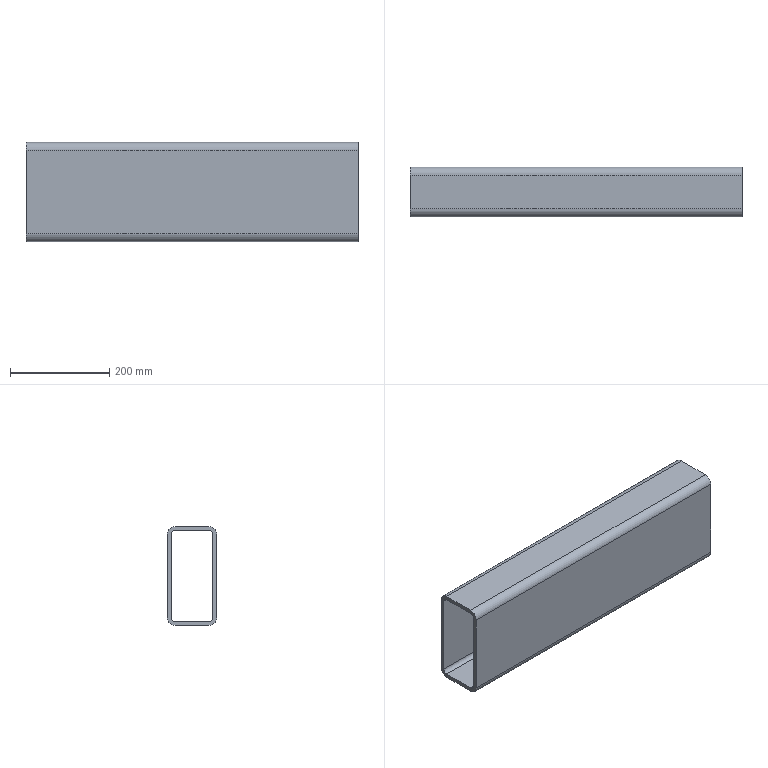Part | STEP file | 03-Longitudinal beam (flat tube 200x100x8)_default<machining> | 1 solid | 18 faces | box 670 x 100 x 200 mm | volume 2934054 mm3 | plane 10 | cylinder 8 | commonest cylinder face diameters 16 x4 32 x4
STEP:
#1=CARTESIAN_POINT('',(0.,0.,0.));
#2=DIRECTION('',(0.,0.,1.));
#3=DIRECTION('',(1.,0.,0.));
#4=AXIS2_PLACEMENT_3D('',#1,#2,#3);
#5=CARTESIAN_POINT('',(0.,50.,84.));
#6=VERTEX_POINT('',#5);
#7=CARTESIAN_POINT('',(0.,34.,100.));
#8=VERTEX_POINT('',#7);
#9=CARTESIAN_POINT('',(0.,34.,84.));
#10=DIRECTION('',(1.,0.,0.));
#11=DIRECTION('',(0.,0.,-1.));
#12=AXIS2_PLACEMENT_3D('',#9,#10,#11);
#13=CIRCLE('',#12,16.);
#14=CARTESIAN_POINT('',(670.,34.,84.));
#15=DIRECTION('',(-1.,0.,0.));
#16=DIRECTION('',(0.,0.,1.));
#17=AXIS2_PLACEMENT_3D('',#14,#15,#16);
#18=CYLINDRICAL_SURFACE('',#17,16.);
#19=CARTESIAN_POINT('',(3.142,670.));
#20=DIRECTION('',(-1.,0.));
#21=VECTOR('',#20,1.);
#22=LINE('',#19,#21);
#23=(GEOMETRIC_REPRESENTATION_CONTEXT(2)PARAMETRIC_REPRESENTATION_CONTEXT()REPRESENTATION_CONTEXT('',''));
#24=DEFINITIONAL_REPRESENTATION('',(#22),#23);
#25=PCURVE('',#18,#24);
#26=CARTESIAN_POINT('',(0.,34.,84.));
#27=DIRECTION('',(1.,0.,0.));
#28=DIRECTION('',(0.,0.,-1.));
#29=AXIS2_PLACEMENT_3D('',#26,#27,#28);
#30=PLANE('',#29);
#31=CARTESIAN_POINT('',(0.,0.));
#32=DIRECTION('',(1.,0.));
#33=AXIS2_PLACEMENT_2D('',#31,#32);
#34=CIRCLE('',#33,16.);
#35=(GEOMETRIC_REPRESENTATION_CONTEXT(2)PARAMETRIC_REPRESENTATION_CONTEXT()REPRESENTATION_CONTEXT('',''));
#36=DEFINITIONAL_REPRESENTATION('',(#34),#35);
#37=PCURVE('',#30,#36);
#38=SURFACE_CURVE('',#13,(#25,#37),.PCURVE_S1.);
#39=EDGE_CURVE('',#6,#8,#38,.T.);
#40=ORIENTED_EDGE('',*,*,#39,.T.);
#41=CARTESIAN_POINT('',(670.,34.,100.));
#42=VERTEX_POINT('',#41);
#43=CARTESIAN_POINT('',(670.,34.,100.));
#44=DIRECTION('',(-1.,0.,0.));
#45=VECTOR('',#44,1.);
#46=LINE('',#43,#45);
#47=CARTESIAN_POINT('',(0.,0.));
#48=DIRECTION('',(0.,1.));
#49=VECTOR('',#48,1.);
#50=LINE('',#47,#49);
#51=(GEOMETRIC_REPRESENTATION_CONTEXT(2)PARAMETRIC_REPRESENTATION_CONTEXT()REPRESENTATION_CONTEXT('',''));
#52=DEFINITIONAL_REPRESENTATION('',(#50),#51);
#53=PCURVE('',#18,#52);
#54=CARTESIAN_POINT('',(670.,34.,100.));
#55=DIRECTION('',(0.,0.,-1.));
#56=DIRECTION('',(-1.,0.,0.));
#57=AXIS2_PLACEMENT_3D('',#54,#55,#56);
#58=PLANE('',#57);
#59=CARTESIAN_POINT('',(0.,0.));
#60=DIRECTION('',(1.,0.));
#61=VECTOR('',#60,1.);
#62=LINE('',#59,#61);
#63=(GEOMETRIC_REPRESENTATION_CONTEXT(2)PARAMETRIC_REPRESENTATION_CONTEXT()REPRESENTATION_CONTEXT('',''));
#64=DEFINITIONAL_REPRESENTATION('',(#62),#63);
#65=PCURVE('',#58,#64);
#66=SURFACE_CURVE('',#46,(#53,#65),.PCURVE_S1.);
#67=EDGE_CURVE('',#42,#8,#66,.T.);
#68=ORIENTED_EDGE('',*,*,#67,.F.);
#69=CARTESIAN_POINT('',(670.,50.,84.));
#70=VERTEX_POINT('',#69);
#71=CARTESIAN_POINT('',(670.,34.,84.));
#72=DIRECTION('',(1.,0.,0.));
#73=DIRECTION('',(0.,0.,-1.));
#74=AXIS2_PLACEMENT_3D('',#71,#72,#73);
#75=CIRCLE('',#74,16.);
#76=CARTESIAN_POINT('',(3.142,0.));
#77=DIRECTION('',(-1.,0.));
#78=VECTOR('',#77,1.);
#79=LINE('',#76,#78);
#80=(GEOMETRIC_REPRESENTATION_CONTEXT(2)PARAMETRIC_REPRESENTATION_CONTEXT()REPRESENTATION_CONTEXT('',''));
#81=DEFINITIONAL_REPRESENTATION('',(#79),#80);
#82=PCURVE('',#18,#81);
#83=CARTESIAN_POINT('',(670.,34.,84.));
#84=DIRECTION('',(1.,0.,0.));
#85=DIRECTION('',(0.,0.,-1.));
#86=AXIS2_PLACEMENT_3D('',#83,#84,#85);
#87=PLANE('',#86);
#88=CARTESIAN_POINT('',(0.,0.));
#89=DIRECTION('',(1.,0.));
#90=AXIS2_PLACEMENT_2D('',#88,#89);
#91=CIRCLE('',#90,16.);
#92=(GEOMETRIC_REPRESENTATION_CONTEXT(2)PARAMETRIC_REPRESENTATION_CONTEXT()REPRESENTATION_CONTEXT('',''));
#93=DEFINITIONAL_REPRESENTATION('',(#91),#92);
#94=PCURVE('',#87,#93);
#95=SURFACE_CURVE('',#75,(#82,#94),.PCURVE_S1.);
#96=EDGE_CURVE('',#70,#42,#95,.T.);
#97=ORIENTED_EDGE('',*,*,#96,.F.);
#98=CARTESIAN_POINT('',(670.,50.,84.));
#99=DIRECTION('',(-1.,0.,0.));
#100=VECTOR('',#99,1.);
#101=LINE('',#98,#100);
#102=CARTESIAN_POINT('',(1.571,0.));
#103=DIRECTION('',(0.,1.));
#104=VECTOR('',#103,1.);
#105=LINE('',#102,#104);
#106=(GEOMETRIC_REPRESENTATION_CONTEXT(2)PARAMETRIC_REPRESENTATION_CONTEXT()REPRESENTATION_CONTEXT('',''));
#107=DEFINITIONAL_REPRESENTATION('',(#105),#106);
#108=PCURVE('',#18,#107);
#109=CARTESIAN_POINT('',(670.,50.,84.));
#110=DIRECTION('',(0.,-1.,0.));
#111=DIRECTION('',(0.,0.,-1.));
#112=AXIS2_PLACEMENT_3D('',#109,#110,#111);
#113=PLANE('',#112);
#114=CARTESIAN_POINT('',(0.,0.));
#115=DIRECTION('',(0.,-1.));
#116=VECTOR('',#115,1.);
#117=LINE('',#114,#116);
#118=(GEOMETRIC_REPRESENTATION_CONTEXT(2)PARAMETRIC_REPRESENTATION_CONTEXT()REPRESENTATION_CONTEXT('',''));
#119=DEFINITIONAL_REPRESENTATION('',(#117),#118);
#120=PCURVE('',#113,#119);
#121=SURFACE_CURVE('',#101,(#108,#120),.PCURVE_S1.);
#122=EDGE_CURVE('',#70,#6,#121,.T.);
#123=ORIENTED_EDGE('',*,*,#122,.T.);
#124=EDGE_LOOP('',(#40,#68,#97,#123));
#125=FACE_BOUND('',#124,.T.);
#126=ADVANCED_FACE('',(#125),#18,.T.);
#127=CARTESIAN_POINT('',(0.,-34.,100.));
#128=VERTEX_POINT('',#127);
#129=CARTESIAN_POINT('',(0.,34.,100.));
#130=DIRECTION('',(0.,-1.,0.));
#131=VECTOR('',#130,1.);
#132=LINE('',#129,#131);
#133=CARTESIAN_POINT('',(670.,0.));
#134=DIRECTION('',(0.,-1.));
#135=VECTOR('',#134,1.);
#136=LINE('',#133,#135);
#137=(GEOMETRIC_REPRESENTATION_CONTEXT(2)PARAMETRIC_REPRESENTATION_CONTEXT()REPRESENTATION_CONTEXT('',''));
#138=DEFINITIONAL_REPRESENTATION('',(#136),#137);
#139=PCURVE('',#58,#138);
#140=CARTESIAN_POINT('',(-16.,0.));
#141=DIRECTION('',(0.,-1.));
#142=VECTOR('',#141,1.);
#143=LINE('',#140,#142);
#144=(GEOMETRIC_REPRESENTATION_CONTEXT(2)PARAMETRIC_REPRESENTATION_CONTEXT()REPRESENTATION_CONTEXT('',''));
#145=DEFINITIONAL_REPRESENTATION('',(#143),#144);
#146=PCURVE('',#30,#145);
#147=SURFACE_CURVE('',#132,(#139,#146),.PCURVE_S1.);
#148=EDGE_CURVE('',#8,#128,#147,.T.);
#149=ORIENTED_EDGE('',*,*,#148,.T.);
#150=CARTESIAN_POINT('',(670.,-34.,100.));
#151=VERTEX_POINT('',#150);
#152=CARTESIAN_POINT('',(670.,-34.,100.));
#153=DIRECTION('',(-1.,0.,0.));
#154=VECTOR('',#153,1.);
#155=LINE('',#152,#154);
#156=CARTESIAN_POINT('',(0.,-68.));
#157=DIRECTION('',(1.,0.));
#158=VECTOR('',#157,1.);
#159=LINE('',#156,#158);
#160=(GEOMETRIC_REPRESENTATION_CONTEXT(2)PARAMETRIC_REPRESENTATION_CONTEXT()REPRESENTATION_CONTEXT('',''));
#161=DEFINITIONAL_REPRESENTATION('',(#159),#160);
#162=PCURVE('',#58,#161);
#163=CARTESIAN_POINT('',(670.,-34.,84.));
#164=DIRECTION('',(-1.,0.,0.));
#165=DIRECTION('',(0.,0.,1.));
#166=AXIS2_PLACEMENT_3D('',#163,#164,#165);
#167=CYLINDRICAL_SURFACE('',#166,16.);
#168=CARTESIAN_POINT('',(6.283,0.));
#169=DIRECTION('',(0.,1.));
#170=VECTOR('',#169,1.);
#171=LINE('',#168,#170);
#172=(GEOMETRIC_REPRESENTATION_CONTEXT(2)PARAMETRIC_REPRESENTATION_CONTEXT()REPRESENTATION_CONTEXT('',''));
#173=DEFINITIONAL_REPRESENTATION('',(#171),#172);
#174=PCURVE('',#167,#173);
#175=SURFACE_CURVE('',#155,(#162,#174),.PCURVE_S1.);
#176=EDGE_CURVE('',#151,#128,#175,.T.);
#177=ORIENTED_EDGE('',*,*,#176,.F.);
#178=CARTESIAN_POINT('',(670.,34.,100.));
#179=DIRECTION('',(0.,-1.,0.));
#180=VECTOR('',#179,1.);
#181=LINE('',#178,#180);
#182=CARTESIAN_POINT('',(0.,0.));
#183=DIRECTION('',(0.,-1.));
#184=VECTOR('',#183,1.);
#185=LINE('',#182,#184);
#186=(GEOMETRIC_REPRESENTATION_CONTEXT(2)PARAMETRIC_REPRESENTATION_CONTEXT()REPRESENTATION_CONTEXT('',''));
#187=DEFINITIONAL_REPRESENTATION('',(#185),#186);
#188=PCURVE('',#58,#187);
#189=CARTESIAN_POINT('',(-16.,0.));
#190=DIRECTION('',(0.,-1.));
#191=VECTOR('',#190,1.);
#192=LINE('',#189,#191);
#193=(GEOMETRIC_REPRESENTATION_CONTEXT(2)PARAMETRIC_REPRESENTATION_CONTEXT()REPRESENTATION_CONTEXT('',''));
#194=DEFINITIONAL_REPRESENTATION('',(#192),#193);
#195=PCURVE('',#87,#194);
#196=SURFACE_CURVE('',#181,(#188,#195),.PCURVE_S1.);
#197=EDGE_CURVE('',#42,#151,#196,.T.);
#198=ORIENTED_EDGE('',*,*,#197,.F.);
#199=ORIENTED_EDGE('',*,*,#67,.T.);
#200=EDGE_LOOP('',(#149,#177,#198,#199));
#201=FACE_BOUND('',#200,.T.);
#202=ADVANCED_FACE('',(#201),#58,.F.);
#203=CARTESIAN_POINT('',(0.,-50.,84.));
#204=VERTEX_POINT('',#203);
#205=CARTESIAN_POINT('',(0.,-34.,84.));
#206=DIRECTION('',(1.,0.,0.));
#207=DIRECTION('',(0.,0.,-1.));
#208=AXIS2_PLACEMENT_3D('',#205,#206,#207);
#209=CIRCLE('',#208,16.);
#210=CARTESIAN_POINT('',(9.425,670.));
#211=DIRECTION('',(-1.,0.));
#212=VECTOR('',#211,1.);
#213=LINE('',#210,#212);
#214=(GEOMETRIC_REPRESENTATION_CONTEXT(2)PARAMETRIC_REPRESENTATION_CONTEXT()REPRESENTATION_CONTEXT('',''));
#215=DEFINITIONAL_REPRESENTATION('',(#213),#214);
#216=PCURVE('',#167,#215);
#217=CARTESIAN_POINT('',(0.,-68.));
#218=DIRECTION('',(1.,0.));
#219=AXIS2_PLACEMENT_2D('',#217,#218);
#220=CIRCLE('',#219,16.);
#221=(GEOMETRIC_REPRESENTATION_CONTEXT(2)PARAMETRIC_REPRESENTATION_CONTEXT()REPRESENTATION_CONTEXT('',''));
#222=DEFINITIONAL_REPRESENTATION('',(#220),#221);
#223=PCURVE('',#30,#222);
#224=SURFACE_CURVE('',#209,(#216,#223),.PCURVE_S1.);
#225=EDGE_CURVE('',#128,#204,#224,.T.);
#226=ORIENTED_EDGE('',*,*,#225,.T.);
#227=CARTESIAN_POINT('',(670.,-50.,84.));
#228=VERTEX_POINT('',#227);
#229=CARTESIAN_POINT('',(670.,-50.,84.));
#230=DIRECTION('',(-1.,0.,0.));
#231=VECTOR('',#230,1.);
#232=LINE('',#229,#231);
#233=CARTESIAN_POINT('',(4.712,0.));
#234=DIRECTION('',(0.,1.));
#235=VECTOR('',#234,1.);
#236=LINE('',#233,#235);
#237=(GEOMETRIC_REPRESENTATION_CONTEXT(2)PARAMETRIC_REPRESENTATION_CONTEXT()REPRESENTATION_CONTEXT('',''));
#238=DEFINITIONAL_REPRESENTATION('',(#236),#237);
#239=PCURVE('',#167,#238);
#240=CARTESIAN_POINT('',(670.,-50.,-84.));
#241=DIRECTION('',(0.,1.,0.));
#242=DIRECTION('',(0.,0.,1.));
#243=AXIS2_PLACEMENT_3D('',#240,#241,#242);
#244=PLANE('',#243);
#245=CARTESIAN_POINT('',(168.,0.));
#246=DIRECTION('',(0.,-1.));
#247=VECTOR('',#246,1.);
#248=LINE('',#245,#247);
#249=(GEOMETRIC_REPRESENTATION_CONTEXT(2)PARAMETRIC_REPRESENTATION_CONTEXT()REPRESENTATION_CONTEXT('',''));
#250=DEFINITIONAL_REPRESENTATION('',(#248),#249);
#251=PCURVE('',#244,#250);
#252=SURFACE_CURVE('',#232,(#239,#251),.PCURVE_S1.);
#253=EDGE_CURVE('',#228,#204,#252,.T.);
#254=ORIENTED_EDGE('',*,*,#253,.F.);
#255=CARTESIAN_POINT('',(670.,-34.,84.));
#256=DIRECTION('',(1.,0.,0.));
#257=DIRECTION('',(0.,0.,-1.));
#258=AXIS2_PLACEMENT_3D('',#255,#256,#257);
#259=CIRCLE('',#258,16.);
#260=CARTESIAN_POINT('',(9.425,0.));
#261=DIRECTION('',(-1.,0.));
#262=VECTOR('',#261,1.);
#263=LINE('',#260,#262);
#264=(GEOMETRIC_REPRESENTATION_CONTEXT(2)PARAMETRIC_REPRESENTATION_CONTEXT()REPRESENTATION_CONTEXT('',''));
#265=DEFINITIONAL_REPRESENTATION('',(#263),#264);
#266=PCURVE('',#167,#265);
#267=CARTESIAN_POINT('',(0.,-68.));
#268=DIRECTION('',(1.,0.));
#269=AXIS2_PLACEMENT_2D('',#267,#268);
#270=CIRCLE('',#269,16.);
#271=(GEOMETRIC_REPRESENTATION_CONTEXT(2)PARAMETRIC_REPRESENTATION_CONTEXT()REPRESENTATION_CONTEXT('',''));
#272=DEFINITIONAL_REPRESENTATION('',(#270),#271);
#273=PCURVE('',#87,#272);
#274=SURFACE_CURVE('',#259,(#266,#273),.PCURVE_S1.);
#275=EDGE_CURVE('',#151,#228,#274,.T.);
#276=ORIENTED_EDGE('',*,*,#275,.F.);
#277=ORIENTED_EDGE('',*,*,#176,.T.);
#278=EDGE_LOOP('',(#226,#254,#276,#277));
#279=FACE_BOUND('',#278,.T.);
#280=ADVANCED_FACE('',(#279),#167,.T.);
#281=CARTESIAN_POINT('',(0.,-50.,-84.));
#282=VERTEX_POINT('',#281);
#283=CARTESIAN_POINT('',(0.,-50.,-84.));
#284=DIRECTION('',(0.,0.,-1.));
#285=VECTOR('',#284,1.);
#286=LINE('',#283,#285);
#287=CARTESIAN_POINT('',(0.,-670.));
#288=DIRECTION('',(-1.,0.));
#289=VECTOR('',#288,1.);
#290=LINE('',#287,#289);
#291=(GEOMETRIC_REPRESENTATION_CONTEXT(2)PARAMETRIC_REPRESENTATION_CONTEXT()REPRESENTATION_CONTEXT('',''));
#292=DEFINITIONAL_REPRESENTATION('',(#290),#291);
#293=PCURVE('',#244,#292);
#294=CARTESIAN_POINT('',(168.,-84.));
#295=DIRECTION('',(1.,0.));
#296=VECTOR('',#295,1.);
#297=LINE('',#294,#296);
#298=(GEOMETRIC_REPRESENTATION_CONTEXT(2)PARAMETRIC_REPRESENTATION_CONTEXT()REPRESENTATION_CONTEXT('',''));
#299=DEFINITIONAL_REPRESENTATION('',(#297),#298);
#300=PCURVE('',#30,#299);
#301=SURFACE_CURVE('',#286,(#293,#300),.PCURVE_S1.);
#302=EDGE_CURVE('',#204,#282,#301,.T.);
#303=ORIENTED_EDGE('',*,*,#302,.T.);
#304=CARTESIAN_POINT('',(670.,-50.,-84.));
#305=VERTEX_POINT('',#304);
#306=CARTESIAN_POINT('',(670.,-50.,-84.));
#307=DIRECTION('',(-1.,0.,0.));
#308=VECTOR('',#307,1.);
#309=LINE('',#306,#308);
#310=CARTESIAN_POINT('',(0.,0.));
#311=DIRECTION('',(0.,-1.));
#312=VECTOR('',#311,1.);
#313=LINE('',#310,#312);
#314=(GEOMETRIC_REPRESENTATION_CONTEXT(2)PARAMETRIC_REPRESENTATION_CONTEXT()REPRESENTATION_CONTEXT('',''));
#315=DEFINITIONAL_REPRESENTATION('',(#313),#314);
#316=PCURVE('',#244,#315);
#317=CARTESIAN_POINT('',(670.,-34.,-84.));
#318=DIRECTION('',(-1.,0.,0.));
#319=DIRECTION('',(0.,0.,1.));
#320=AXIS2_PLACEMENT_3D('',#317,#318,#319);
#321=CYLINDRICAL_SURFACE('',#320,16.);
#322=CARTESIAN_POINT('',(4.712,0.));
#323=DIRECTION('',(0.,1.));
#324=VECTOR('',#323,1.);
#325=LINE('',#322,#324);
#326=(GEOMETRIC_REPRESENTATION_CONTEXT(2)PARAMETRIC_REPRESENTATION_CONTEXT()REPRESENTATION_CONTEXT('',''));
#327=DEFINITIONAL_REPRESENTATION('',(#325),#326);
#328=PCURVE('',#321,#327);
#329=SURFACE_CURVE('',#309,(#316,#328),.PCURVE_S1.);
#330=EDGE_CURVE('',#305,#282,#329,.T.);
#331=ORIENTED_EDGE('',*,*,#330,.F.);
#332=CARTESIAN_POINT('',(670.,-50.,-84.));
#333=DIRECTION('',(0.,0.,-1.));
#334=VECTOR('',#333,1.);
#335=LINE('',#332,#334);
#336=CARTESIAN_POINT('',(0.,0.));
#337=DIRECTION('',(-1.,0.));
#338=VECTOR('',#337,1.);
#339=LINE('',#336,#338);
#340=(GEOMETRIC_REPRESENTATION_CONTEXT(2)PARAMETRIC_REPRESENTATION_CONTEXT()REPRESENTATION_CONTEXT('',''));
#341=DEFINITIONAL_REPRESENTATION('',(#339),#340);
#342=PCURVE('',#244,#341);
#343=CARTESIAN_POINT('',(168.,-84.));
#344=DIRECTION('',(1.,0.));
#345=VECTOR('',#344,1.);
#346=LINE('',#343,#345);
#347=(GEOMETRIC_REPRESENTATION_CONTEXT(2)PARAMETRIC_REPRESENTATION_CONTEXT()REPRESENTATION_CONTEXT('',''));
#348=DEFINITIONAL_REPRESENTATION('',(#346),#347);
#349=PCURVE('',#87,#348);
#350=SURFACE_CURVE('',#335,(#342,#349),.PCURVE_S1.);
#351=EDGE_CURVE('',#228,#305,#350,.T.);
#352=ORIENTED_EDGE('',*,*,#351,.F.);
#353=ORIENTED_EDGE('',*,*,#253,.T.);
#354=EDGE_LOOP('',(#303,#331,#352,#353));
#355=FACE_BOUND('',#354,.T.);
#356=ADVANCED_FACE('',(#355),#244,.F.);
#357=CARTESIAN_POINT('',(0.,-34.,-100.));
#358=VERTEX_POINT('',#357);
#359=CARTESIAN_POINT('',(0.,-34.,-84.));
#360=DIRECTION('',(1.,0.,0.));
#361=DIRECTION('',(0.,0.,-1.));
#362=AXIS2_PLACEMENT_3D('',#359,#360,#361);
#363=CIRCLE('',#362,16.);
#364=CARTESIAN_POINT('',(9.425,670.));
#365=DIRECTION('',(-1.,0.));
#366=VECTOR('',#365,1.);
#367=LINE('',#364,#366);
#368=(GEOMETRIC_REPRESENTATION_CONTEXT(2)PARAMETRIC_REPRESENTATION_CONTEXT()REPRESENTATION_CONTEXT('',''));
#369=DEFINITIONAL_REPRESENTATION('',(#367),#368);
#370=PCURVE('',#321,#369);
#371=CARTESIAN_POINT('',(168.,-68.));
#372=DIRECTION('',(1.,0.));
#373=AXIS2_PLACEMENT_2D('',#371,#372);
#374=CIRCLE('',#373,16.);
#375=(GEOMETRIC_REPRESENTATION_CONTEXT(2)PARAMETRIC_REPRESENTATION_CONTEXT()REPRESENTATION_CONTEXT('',''));
#376=DEFINITIONAL_REPRESENTATION('',(#374),#375);
#377=PCURVE('',#30,#376);
#378=SURFACE_CURVE('',#363,(#370,#377),.PCURVE_S1.);
#379=EDGE_CURVE('',#282,#358,#378,.T.);
#380=ORIENTED_EDGE('',*,*,#379,.T.);
#381=CARTESIAN_POINT('',(670.,-34.,-100.));
#382=VERTEX_POINT('',#381);
#383=CARTESIAN_POINT('',(670.,-34.,-100.));
#384=DIRECTION('',(-1.,0.,0.));
#385=VECTOR('',#384,1.);
#386=LINE('',#383,#385);
#387=CARTESIAN_POINT('',(3.142,0.));
#388=DIRECTION('',(0.,1.));
#389=VECTOR('',#388,1.);
#390=LINE('',#387,#389);
#391=(GEOMETRIC_REPRESENTATION_CONTEXT(2)PARAMETRIC_REPRESENTATION_CONTEXT()REPRESENTATION_CONTEXT('',''));
#392=DEFINITIONAL_REPRESENTATION('',(#390),#391);
#393=PCURVE('',#321,#392);
#394=CARTESIAN_POINT('',(670.,-34.,-100.));
#395=DIRECTION('',(0.,0.,1.));
#396=DIRECTION('',(1.,0.,0.));
#397=AXIS2_PLACEMENT_3D('',#394,#395,#396);
#398=PLANE('',#397);
#399=CARTESIAN_POINT('',(0.,0.));
#400=DIRECTION('',(-1.,0.));
#401=VECTOR('',#400,1.);
#402=LINE('',#399,#401);
#403=(GEOMETRIC_REPRESENTATION_CONTEXT(2)PARAMETRIC_REPRESENTATION_CONTEXT()REPRESENTATION_CONTEXT('',''));
#404=DEFINITIONAL_REPRESENTATION('',(#402),#403);
#405=PCURVE('',#398,#404);
#406=SURFACE_CURVE('',#386,(#393,#405),.PCURVE_S1.);
#407=EDGE_CURVE('',#382,#358,#406,.T.);
#408=ORIENTED_EDGE('',*,*,#407,.F.);
#409=CARTESIAN_POINT('',(670.,-34.,-84.));
#410=DIRECTION('',(1.,0.,0.));
#411=DIRECTION('',(0.,0.,-1.));
#412=AXIS2_PLACEMENT_3D('',#409,#410,#411);
#413=CIRCLE('',#412,16.);
#414=CARTESIAN_POINT('',(9.425,0.));
#415=DIRECTION('',(-1.,0.));
#416=VECTOR('',#415,1.);
#417=LINE('',#414,#416);
#418=(GEOMETRIC_REPRESENTATION_CONTEXT(2)PARAMETRIC_REPRESENTATION_CONTEXT()REPRESENTATION_CONTEXT('',''));
#419=DEFINITIONAL_REPRESENTATION('',(#417),#418);
#420=PCURVE('',#321,#419);
#421=CARTESIAN_POINT('',(168.,-68.));
#422=DIRECTION('',(1.,0.));
#423=AXIS2_PLACEMENT_2D('',#421,#422);
#424=CIRCLE('',#423,16.);
#425=(GEOMETRIC_REPRESENTATION_CONTEXT(2)PARAMETRIC_REPRESENTATION_CONTEXT()REPRESENTATION_CONTEXT('',''));
#426=DEFINITIONAL_REPRESENTATION('',(#424),#425);
#427=PCURVE('',#87,#426);
#428=SURFACE_CURVE('',#413,(#420,#427),.PCURVE_S1.);
#429=EDGE_CURVE('',#305,#382,#428,.T.);
#430=ORIENTED_EDGE('',*,*,#429,.F.);
#431=ORIENTED_EDGE('',*,*,#330,.T.);
#432=EDGE_LOOP('',(#380,#408,#430,#431));
#433=FACE_BOUND('',#432,.T.);
#434=ADVANCED_FACE('',(#433),#321,.T.);
#435=CARTESIAN_POINT('',(0.,34.,-100.));
#436=VERTEX_POINT('',#435);
#437=CARTESIAN_POINT('',(0.,-34.,-100.));
#438=DIRECTION('',(0.,1.,0.));
#439=VECTOR('',#438,1.);
#440=LINE('',#437,#439);
#441=CARTESIAN_POINT('',(-670.,0.));
#442=DIRECTION('',(0.,1.));
#443=VECTOR('',#442,1.);
#444=LINE('',#441,#443);
#445=(GEOMETRIC_REPRESENTATION_CONTEXT(2)PARAMETRIC_REPRESENTATION_CONTEXT()REPRESENTATION_CONTEXT('',''));
#446=DEFINITIONAL_REPRESENTATION('',(#444),#445);
#447=PCURVE('',#398,#446);
#448=CARTESIAN_POINT('',(184.,-68.));
#449=DIRECTION('',(0.,1.));
#450=VECTOR('',#449,1.);
#451=LINE('',#448,#450);
#452=(GEOMETRIC_REPRESENTATION_CONTEXT(2)PARAMETRIC_REPRESENTATION_CONTEXT()REPRESENTATION_CONTEXT('',''));
#453=DEFINITIONAL_REPRESENTATION('',(#451),#452);
#454=PCURVE('',#30,#453);
#455=SURFACE_CURVE('',#440,(#447,#454),.PCURVE_S1.);
#456=EDGE_CURVE('',#358,#436,#455,.T.);
#457=ORIENTED_EDGE('',*,*,#456,.T.);
#458=CARTESIAN_POINT('',(670.,34.,-100.));
#459=VERTEX_POINT('',#458);
#460=CARTESIAN_POINT('',(670.,34.,-100.));
#461=DIRECTION('',(-1.,0.,0.));
#462=VECTOR('',#461,1.);
#463=LINE('',#460,#462);
#464=CARTESIAN_POINT('',(0.,68.));
#465=DIRECTION('',(-1.,0.));
#466=VECTOR('',#465,1.);
#467=LINE('',#464,#466);
#468=(GEOMETRIC_REPRESENTATION_CONTEXT(2)PARAMETRIC_REPRESENTATION_CONTEXT()REPRESENTATION_CONTEXT('',''));
#469=DEFINITIONAL_REPRESENTATION('',(#467),#468);
#470=PCURVE('',#398,#469);
#471=CARTESIAN_POINT('',(670.,34.,-84.));
#472=DIRECTION('',(-1.,0.,0.));
#473=DIRECTION('',(0.,0.,1.));
#474=AXIS2_PLACEMENT_3D('',#471,#472,#473);
#475=CYLINDRICAL_SURFACE('',#474,16.);
#476=CARTESIAN_POINT('',(3.142,0.));
#477=DIRECTION('',(0.,1.));
#478=VECTOR('',#477,1.);
#479=LINE('',#476,#478);
#480=(GEOMETRIC_REPRESENTATION_CONTEXT(2)PARAMETRIC_REPRESENTATION_CONTEXT()REPRESENTATION_CONTEXT('',''));
#481=DEFINITIONAL_REPRESENTATION('',(#479),#480);
#482=PCURVE('',#475,#481);
#483=SURFACE_CURVE('',#463,(#470,#482),.PCURVE_S1.);
#484=EDGE_CURVE('',#459,#436,#483,.T.);
#485=ORIENTED_EDGE('',*,*,#484,.F.);
#486=CARTESIAN_POINT('',(670.,-34.,-100.));
#487=DIRECTION('',(0.,1.,0.));
#488=VECTOR('',#487,1.);
#489=LINE('',#486,#488);
#490=CARTESIAN_POINT('',(0.,0.));
#491=DIRECTION('',(0.,1.));
#492=VECTOR('',#491,1.);
#493=LINE('',#490,#492);
#494=(GEOMETRIC_REPRESENTATION_CONTEXT(2)PARAMETRIC_REPRESENTATION_CONTEXT()REPRESENTATION_CONTEXT('',''));
#495=DEFINITIONAL_REPRESENTATION('',(#493),#494);
#496=PCURVE('',#398,#495);
#497=CARTESIAN_POINT('',(184.,-68.));
#498=DIRECTION('',(0.,1.));
#499=VECTOR('',#498,1.);
#500=LINE('',#497,#499);
#501=(GEOMETRIC_REPRESENTATION_CONTEXT(2)PARAMETRIC_REPRESENTATION_CONTEXT()REPRESENTATION_CONTEXT('',''));
#502=DEFINITIONAL_REPRESENTATION('',(#500),#501);
#503=PCURVE('',#87,#502);
#504=SURFACE_CURVE('',#489,(#496,#503),.PCURVE_S1.);
#505=EDGE_CURVE('',#382,#459,#504,.T.);
#506=ORIENTED_EDGE('',*,*,#505,.F.);
#507=ORIENTED_EDGE('',*,*,#407,.T.);
#508=EDGE_LOOP('',(#457,#485,#506,#507));
#509=FACE_BOUND('',#508,.T.);
#510=ADVANCED_FACE('',(#509),#398,.F.);
#511=CARTESIAN_POINT('',(0.,50.,-84.));
#512=VERTEX_POINT('',#511);
#513=CARTESIAN_POINT('',(0.,34.,-84.));
#514=DIRECTION('',(1.,0.,0.));
#515=DIRECTION('',(0.,0.,-1.));
#516=AXIS2_PLACEMENT_3D('',#513,#514,#515);
#517=CIRCLE('',#516,16.);
#518=CARTESIAN_POINT('',(3.142,670.));
#519=DIRECTION('',(-1.,0.));
#520=VECTOR('',#519,1.);
#521=LINE('',#518,#520);
#522=(GEOMETRIC_REPRESENTATION_CONTEXT(2)PARAMETRIC_REPRESENTATION_CONTEXT()REPRESENTATION_CONTEXT('',''));
#523=DEFINITIONAL_REPRESENTATION('',(#521),#522);
#524=PCURVE('',#475,#523);
#525=CARTESIAN_POINT('',(168.,0.));
#526=DIRECTION('',(1.,0.));
#527=AXIS2_PLACEMENT_2D('',#525,#526);
#528=CIRCLE('',#527,16.);
#529=(GEOMETRIC_REPRESENTATION_CONTEXT(2)PARAMETRIC_REPRESENTATION_CONTEXT()REPRESENTATION_CONTEXT('',''));
#530=DEFINITIONAL_REPRESENTATION('',(#528),#529);
#531=PCURVE('',#30,#530);
#532=SURFACE_CURVE('',#517,(#524,#531),.PCURVE_S1.);
#533=EDGE_CURVE('',#436,#512,#532,.T.);
#534=ORIENTED_EDGE('',*,*,#533,.T.);
#535=CARTESIAN_POINT('',(670.,50.,-84.));
#536=VERTEX_POINT('',#535);
#537=CARTESIAN_POINT('',(670.,50.,-84.));
#538=DIRECTION('',(-1.,0.,0.));
#539=VECTOR('',#538,1.);
#540=LINE('',#537,#539);
#541=CARTESIAN_POINT('',(1.571,0.));
#542=DIRECTION('',(0.,1.));
#543=VECTOR('',#542,1.);
#544=LINE('',#541,#543);
#545=(GEOMETRIC_REPRESENTATION_CONTEXT(2)PARAMETRIC_REPRESENTATION_CONTEXT()REPRESENTATION_CONTEXT('',''));
#546=DEFINITIONAL_REPRESENTATION('',(#544),#545);
#547=PCURVE('',#475,#546);
#548=CARTESIAN_POINT('',(168.,0.));
#549=DIRECTION('',(0.,-1.));
#550=VECTOR('',#549,1.);
#551=LINE('',#548,#550);
#552=(GEOMETRIC_REPRESENTATION_CONTEXT(2)PARAMETRIC_REPRESENTATION_CONTEXT()REPRESENTATION_CONTEXT('',''));
#553=DEFINITIONAL_REPRESENTATION('',(#551),#552);
#554=PCURVE('',#113,#553);
#555=SURFACE_CURVE('',#540,(#547,#554),.PCURVE_S1.);
#556=EDGE_CURVE('',#536,#512,#555,.T.);
#557=ORIENTED_EDGE('',*,*,#556,.F.);
#558=CARTESIAN_POINT('',(670.,34.,-84.));
#559=DIRECTION('',(1.,0.,0.));
#560=DIRECTION('',(0.,0.,-1.));
#561=AXIS2_PLACEMENT_3D('',#558,#559,#560);
#562=CIRCLE('',#561,16.);
#563=CARTESIAN_POINT('',(3.142,0.));
#564=DIRECTION('',(-1.,0.));
#565=VECTOR('',#564,1.);
#566=LINE('',#563,#565);
#567=(GEOMETRIC_REPRESENTATION_CONTEXT(2)PARAMETRIC_REPRESENTATION_CONTEXT()REPRESENTATION_CONTEXT('',''));
#568=DEFINITIONAL_REPRESENTATION('',(#566),#567);
#569=PCURVE('',#475,#568);
#570=CARTESIAN_POINT('',(168.,0.));
#571=DIRECTION('',(1.,0.));
#572=AXIS2_PLACEMENT_2D('',#570,#571);
#573=CIRCLE('',#572,16.);
#574=(GEOMETRIC_REPRESENTATION_CONTEXT(2)PARAMETRIC_REPRESENTATION_CONTEXT()REPRESENTATION_CONTEXT('',''));
#575=DEFINITIONAL_REPRESENTATION('',(#573),#574);
#576=PCURVE('',#87,#575);
#577=SURFACE_CURVE('',#562,(#569,#576),.PCURVE_S1.);
#578=EDGE_CURVE('',#459,#536,#577,.T.);
#579=ORIENTED_EDGE('',*,*,#578,.F.);
#580=ORIENTED_EDGE('',*,*,#484,.T.);
#581=EDGE_LOOP('',(#534,#557,#579,#580));
#582=FACE_BOUND('',#581,.T.);
#583=ADVANCED_FACE('',(#582),#475,.T.);
#584=CARTESIAN_POINT('',(670.,-42.,84.));
#585=VERTEX_POINT('',#584);
#586=CARTESIAN_POINT('',(0.,-42.,84.));
#587=VERTEX_POINT('',#586);
#588=CARTESIAN_POINT('',(670.,-42.,84.));
#589=DIRECTION('',(-1.,0.,0.));
#590=VECTOR('',#589,1.);
#591=LINE('',#588,#590);
#592=CARTESIAN_POINT('',(670.,-34.,84.));
#593=DIRECTION('',(-1.,0.,0.));
#594=DIRECTION('',(0.,0.,1.));
#595=AXIS2_PLACEMENT_3D('',#592,#593,#594);
#596=CYLINDRICAL_SURFACE('',#595,8.);
#597=CARTESIAN_POINT('',(4.712,0.));
#598=DIRECTION('',(0.,1.));
#599=VECTOR('',#598,1.);
#600=LINE('',#597,#599);
#601=(GEOMETRIC_REPRESENTATION_CONTEXT(2)PARAMETRIC_REPRESENTATION_CONTEXT()REPRESENTATION_CONTEXT('',''));
#602=DEFINITIONAL_REPRESENTATION('',(#600),#601);
#603=PCURVE('',#596,#602);
#604=CARTESIAN_POINT('',(670.,-42.,-84.));
#605=DIRECTION('',(0.,1.,0.));
#606=DIRECTION('',(0.,0.,1.));
#607=AXIS2_PLACEMENT_3D('',#604,#605,#606);
#608=PLANE('',#607);
#609=CARTESIAN_POINT('',(168.,0.));
#610=DIRECTION('',(0.,-1.));
#611=VECTOR('',#610,1.);
#612=LINE('',#609,#611);
#613=(GEOMETRIC_REPRESENTATION_CONTEXT(2)PARAMETRIC_REPRESENTATION_CONTEXT()REPRESENTATION_CONTEXT('',''));
#614=DEFINITIONAL_REPRESENTATION('',(#612),#613);
#615=PCURVE('',#608,#614);
#616=SURFACE_CURVE('',#591,(#603,#615),.PCURVE_S1.);
#617=EDGE_CURVE('',#585,#587,#616,.T.);
#618=ORIENTED_EDGE('',*,*,#617,.F.);
#619=CARTESIAN_POINT('',(670.,-34.,92.));
#620=VERTEX_POINT('',#619);
#621=CARTESIAN_POINT('',(670.,-34.,84.));
#622=DIRECTION('',(1.,0.,0.));
#623=DIRECTION('',(0.,0.,-1.));
#624=AXIS2_PLACEMENT_3D('',#621,#622,#623);
#625=CIRCLE('',#624,8.);
#626=CARTESIAN_POINT('',(9.425,0.));
#627=DIRECTION('',(-1.,0.));
#628=VECTOR('',#627,1.);
#629=LINE('',#626,#628);
#630=(GEOMETRIC_REPRESENTATION_CONTEXT(2)PARAMETRIC_REPRESENTATION_CONTEXT()REPRESENTATION_CONTEXT('',''));
#631=DEFINITIONAL_REPRESENTATION('',(#629),#630);
#632=PCURVE('',#596,#631);
#633=CARTESIAN_POINT('',(0.,-68.));
#634=DIRECTION('',(1.,0.));
#635=AXIS2_PLACEMENT_2D('',#633,#634);
#636=CIRCLE('',#635,8.);
#637=(GEOMETRIC_REPRESENTATION_CONTEXT(2)PARAMETRIC_REPRESENTATION_CONTEXT()REPRESENTATION_CONTEXT('',''));
#638=DEFINITIONAL_REPRESENTATION('',(#636),#637);
#639=PCURVE('',#87,#638);
#640=SURFACE_CURVE('',#625,(#632,#639),.PCURVE_S1.);
#641=EDGE_CURVE('',#620,#585,#640,.T.);
#642=ORIENTED_EDGE('',*,*,#641,.F.);
#643=CARTESIAN_POINT('',(0.,-34.,92.));
#644=VERTEX_POINT('',#643);
#645=CARTESIAN_POINT('',(670.,-34.,92.));
#646=DIRECTION('',(-1.,0.,0.));
#647=VECTOR('',#646,1.);
#648=LINE('',#645,#647);
#649=CARTESIAN_POINT('',(6.283,0.));
#650=DIRECTION('',(0.,1.));
#651=VECTOR('',#650,1.);
#652=LINE('',#649,#651);
#653=(GEOMETRIC_REPRESENTATION_CONTEXT(2)PARAMETRIC_REPRESENTATION_CONTEXT()REPRESENTATION_CONTEXT('',''));
#654=DEFINITIONAL_REPRESENTATION('',(#652),#653);
#655=PCURVE('',#596,#654);
#656=CARTESIAN_POINT('',(670.,34.,92.));
#657=DIRECTION('',(0.,0.,-1.));
#658=DIRECTION('',(-1.,0.,0.));
#659=AXIS2_PLACEMENT_3D('',#656,#657,#658);
#660=PLANE('',#659);
#661=CARTESIAN_POINT('',(0.,-68.));
#662=DIRECTION('',(1.,0.));
#663=VECTOR('',#662,1.);
#664=LINE('',#661,#663);
#665=(GEOMETRIC_REPRESENTATION_CONTEXT(2)PARAMETRIC_REPRESENTATION_CONTEXT()REPRESENTATION_CONTEXT('',''));
#666=DEFINITIONAL_REPRESENTATION('',(#664),#665);
#667=PCURVE('',#660,#666);
#668=SURFACE_CURVE('',#648,(#655,#667),.PCURVE_S1.);
#669=EDGE_CURVE('',#620,#644,#668,.T.);
#670=ORIENTED_EDGE('',*,*,#669,.T.);
#671=CARTESIAN_POINT('',(0.,-34.,84.));
#672=DIRECTION('',(1.,0.,0.));
#673=DIRECTION('',(0.,0.,-1.));
#674=AXIS2_PLACEMENT_3D('',#671,#672,#673);
#675=CIRCLE('',#674,8.);
#676=CARTESIAN_POINT('',(9.425,670.));
#677=DIRECTION('',(-1.,0.));
#678=VECTOR('',#677,1.);
#679=LINE('',#676,#678);
#680=(GEOMETRIC_REPRESENTATION_CONTEXT(2)PARAMETRIC_REPRESENTATION_CONTEXT()REPRESENTATION_CONTEXT('',''));
#681=DEFINITIONAL_REPRESENTATION('',(#679),#680);
#682=PCURVE('',#596,#681);
#683=CARTESIAN_POINT('',(0.,-68.));
#684=DIRECTION('',(1.,0.));
#685=AXIS2_PLACEMENT_2D('',#683,#684);
#686=CIRCLE('',#685,8.);
#687=(GEOMETRIC_REPRESENTATION_CONTEXT(2)PARAMETRIC_REPRESENTATION_CONTEXT()REPRESENTATION_CONTEXT('',''));
#688=DEFINITIONAL_REPRESENTATION('',(#686),#687);
#689=PCURVE('',#30,#688);
#690=SURFACE_CURVE('',#675,(#682,#689),.PCURVE_S1.);
#691=EDGE_CURVE('',#644,#587,#690,.T.);
#692=ORIENTED_EDGE('',*,*,#691,.T.);
#693=EDGE_LOOP('',(#618,#642,#670,#692));
#694=FACE_BOUND('',#693,.F.);
#695=ADVANCED_FACE('',(#694),#596,.F.);
#696=CARTESIAN_POINT('',(0.,34.,92.));
#697=VERTEX_POINT('',#696);
#698=CARTESIAN_POINT('',(0.,34.,92.));
#699=DIRECTION('',(0.,-1.,0.));
#700=VECTOR('',#699,1.);
#701=LINE('',#698,#700);
#702=CARTESIAN_POINT('',(670.,0.));
#703=DIRECTION('',(0.,-1.));
#704=VECTOR('',#703,1.);
#705=LINE('',#702,#704);
#706=(GEOMETRIC_REPRESENTATION_CONTEXT(2)PARAMETRIC_REPRESENTATION_CONTEXT()REPRESENTATION_CONTEXT('',''));
#707=DEFINITIONAL_REPRESENTATION('',(#705),#706);
#708=PCURVE('',#660,#707);
#709=CARTESIAN_POINT('',(-8.,0.));
#710=DIRECTION('',(0.,-1.));
#711=VECTOR('',#710,1.);
#712=LINE('',#709,#711);
#713=(GEOMETRIC_REPRESENTATION_CONTEXT(2)PARAMETRIC_REPRESENTATION_CONTEXT()REPRESENTATION_CONTEXT('',''));
#714=DEFINITIONAL_REPRESENTATION('',(#712),#713);
#715=PCURVE('',#30,#714);
#716=SURFACE_CURVE('',#701,(#708,#715),.PCURVE_S1.);
#717=EDGE_CURVE('',#697,#644,#716,.T.);
#718=ORIENTED_EDGE('',*,*,#717,.F.);
#719=CARTESIAN_POINT('',(670.,34.,92.));
#720=VERTEX_POINT('',#719);
#721=CARTESIAN_POINT('',(670.,34.,92.));
#722=DIRECTION('',(-1.,0.,0.));
#723=VECTOR('',#722,1.);
#724=LINE('',#721,#723);
#725=CARTESIAN_POINT('',(0.,0.));
#726=DIRECTION('',(1.,0.));
#727=VECTOR('',#726,1.);
#728=LINE('',#725,#727);
#729=(GEOMETRIC_REPRESENTATION_CONTEXT(2)PARAMETRIC_REPRESENTATION_CONTEXT()REPRESENTATION_CONTEXT('',''));
#730=DEFINITIONAL_REPRESENTATION('',(#728),#729);
#731=PCURVE('',#660,#730);
#732=CARTESIAN_POINT('',(670.,34.,84.));
#733=DIRECTION('',(-1.,0.,0.));
#734=DIRECTION('',(0.,0.,1.));
#735=AXIS2_PLACEMENT_3D('',#732,#733,#734);
#736=CYLINDRICAL_SURFACE('',#735,8.);
#737=CARTESIAN_POINT('',(0.,0.));
#738=DIRECTION('',(0.,1.));
#739=VECTOR('',#738,1.);
#740=LINE('',#737,#739);
#741=(GEOMETRIC_REPRESENTATION_CONTEXT(2)PARAMETRIC_REPRESENTATION_CONTEXT()REPRESENTATION_CONTEXT('',''));
#742=DEFINITIONAL_REPRESENTATION('',(#740),#741);
#743=PCURVE('',#736,#742);
#744=SURFACE_CURVE('',#724,(#731,#743),.PCURVE_S1.);
#745=EDGE_CURVE('',#720,#697,#744,.T.);
#746=ORIENTED_EDGE('',*,*,#745,.F.);
#747=CARTESIAN_POINT('',(670.,34.,92.));
#748=DIRECTION('',(0.,-1.,0.));
#749=VECTOR('',#748,1.);
#750=LINE('',#747,#749);
#751=CARTESIAN_POINT('',(0.,0.));
#752=DIRECTION('',(0.,-1.));
#753=VECTOR('',#752,1.);
#754=LINE('',#751,#753);
#755=(GEOMETRIC_REPRESENTATION_CONTEXT(2)PARAMETRIC_REPRESENTATION_CONTEXT()REPRESENTATION_CONTEXT('',''));
#756=DEFINITIONAL_REPRESENTATION('',(#754),#755);
#757=PCURVE('',#660,#756);
#758=CARTESIAN_POINT('',(-8.,0.));
#759=DIRECTION('',(0.,-1.));
#760=VECTOR('',#759,1.);
#761=LINE('',#758,#760);
#762=(GEOMETRIC_REPRESENTATION_CONTEXT(2)PARAMETRIC_REPRESENTATION_CONTEXT()REPRESENTATION_CONTEXT('',''));
#763=DEFINITIONAL_REPRESENTATION('',(#761),#762);
#764=PCURVE('',#87,#763);
#765=SURFACE_CURVE('',#750,(#757,#764),.PCURVE_S1.);
#766=EDGE_CURVE('',#720,#620,#765,.T.);
#767=ORIENTED_EDGE('',*,*,#766,.T.);
#768=ORIENTED_EDGE('',*,*,#669,.T.);
#769=EDGE_LOOP('',(#718,#746,#767,#768));
#770=FACE_BOUND('',#769,.T.);
#771=ADVANCED_FACE('',(#770),#660,.T.);
#772=ORIENTED_EDGE('',*,*,#745,.F.);
#773=CARTESIAN_POINT('',(670.,42.,84.));
#774=VERTEX_POINT('',#773);
#775=CARTESIAN_POINT('',(670.,34.,84.));
#776=DIRECTION('',(1.,0.,0.));
#777=DIRECTION('',(0.,0.,-1.));
#778=AXIS2_PLACEMENT_3D('',#775,#776,#777);
#779=CIRCLE('',#778,8.);
#780=CARTESIAN_POINT('',(3.142,0.));
#781=DIRECTION('',(-1.,0.));
#782=VECTOR('',#781,1.);
#783=LINE('',#780,#782);
#784=(GEOMETRIC_REPRESENTATION_CONTEXT(2)PARAMETRIC_REPRESENTATION_CONTEXT()REPRESENTATION_CONTEXT('',''));
#785=DEFINITIONAL_REPRESENTATION('',(#783),#784);
#786=PCURVE('',#736,#785);
#787=CARTESIAN_POINT('',(0.,0.));
#788=DIRECTION('',(1.,0.));
#789=AXIS2_PLACEMENT_2D('',#787,#788);
#790=CIRCLE('',#789,8.);
#791=(GEOMETRIC_REPRESENTATION_CONTEXT(2)PARAMETRIC_REPRESENTATION_CONTEXT()REPRESENTATION_CONTEXT('',''));
#792=DEFINITIONAL_REPRESENTATION('',(#790),#791);
#793=PCURVE('',#87,#792);
#794=SURFACE_CURVE('',#779,(#786,#793),.PCURVE_S1.);
#795=EDGE_CURVE('',#774,#720,#794,.T.);
#796=ORIENTED_EDGE('',*,*,#795,.F.);
#797=CARTESIAN_POINT('',(0.,42.,84.));
#798=VERTEX_POINT('',#797);
#799=CARTESIAN_POINT('',(670.,42.,84.));
#800=DIRECTION('',(-1.,0.,0.));
#801=VECTOR('',#800,1.);
#802=LINE('',#799,#801);
#803=CARTESIAN_POINT('',(1.571,0.));
#804=DIRECTION('',(0.,1.));
#805=VECTOR('',#804,1.);
#806=LINE('',#803,#805);
#807=(GEOMETRIC_REPRESENTATION_CONTEXT(2)PARAMETRIC_REPRESENTATION_CONTEXT()REPRESENTATION_CONTEXT('',''));
#808=DEFINITIONAL_REPRESENTATION('',(#806),#807);
#809=PCURVE('',#736,#808);
#810=CARTESIAN_POINT('',(670.,42.,84.));
#811=DIRECTION('',(0.,-1.,0.));
#812=DIRECTION('',(0.,0.,-1.));
#813=AXIS2_PLACEMENT_3D('',#810,#811,#812);
#814=PLANE('',#813);
#815=CARTESIAN_POINT('',(0.,0.));
#816=DIRECTION('',(0.,-1.));
#817=VECTOR('',#816,1.);
#818=LINE('',#815,#817);
#819=(GEOMETRIC_REPRESENTATION_CONTEXT(2)PARAMETRIC_REPRESENTATION_CONTEXT()REPRESENTATION_CONTEXT('',''));
#820=DEFINITIONAL_REPRESENTATION('',(#818),#819);
#821=PCURVE('',#814,#820);
#822=SURFACE_CURVE('',#802,(#809,#821),.PCURVE_S1.);
#823=EDGE_CURVE('',#774,#798,#822,.T.);
#824=ORIENTED_EDGE('',*,*,#823,.T.);
#825=CARTESIAN_POINT('',(0.,34.,84.));
#826=DIRECTION('',(1.,0.,0.));
#827=DIRECTION('',(0.,0.,-1.));
#828=AXIS2_PLACEMENT_3D('',#825,#826,#827);
#829=CIRCLE('',#828,8.);
#830=CARTESIAN_POINT('',(3.142,670.));
#831=DIRECTION('',(-1.,0.));
#832=VECTOR('',#831,1.);
#833=LINE('',#830,#832);
#834=(GEOMETRIC_REPRESENTATION_CONTEXT(2)PARAMETRIC_REPRESENTATION_CONTEXT()REPRESENTATION_CONTEXT('',''));
#835=DEFINITIONAL_REPRESENTATION('',(#833),#834);
#836=PCURVE('',#736,#835);
#837=CARTESIAN_POINT('',(0.,0.));
#838=DIRECTION('',(1.,0.));
#839=AXIS2_PLACEMENT_2D('',#837,#838);
#840=CIRCLE('',#839,8.);
#841=(GEOMETRIC_REPRESENTATION_CONTEXT(2)PARAMETRIC_REPRESENTATION_CONTEXT()REPRESENTATION_CONTEXT('',''));
#842=DEFINITIONAL_REPRESENTATION('',(#840),#841);
#843=PCURVE('',#30,#842);
#844=SURFACE_CURVE('',#829,(#836,#843),.PCURVE_S1.);
#845=EDGE_CURVE('',#798,#697,#844,.T.);
#846=ORIENTED_EDGE('',*,*,#845,.T.);
#847=EDGE_LOOP('',(#772,#796,#824,#846));
#848=FACE_BOUND('',#847,.F.);
#849=ADVANCED_FACE('',(#848),#736,.F.);
#850=CARTESIAN_POINT('',(0.,42.,-84.));
#851=VERTEX_POINT('',#850);
#852=CARTESIAN_POINT('',(0.,42.,84.));
#853=DIRECTION('',(0.,0.,1.));
#854=VECTOR('',#853,1.);
#855=LINE('',#852,#854);
#856=CARTESIAN_POINT('',(0.,-670.));
#857=DIRECTION('',(-1.,0.));
#858=VECTOR('',#857,1.);
#859=LINE('',#856,#858);
#860=(GEOMETRIC_REPRESENTATION_CONTEXT(2)PARAMETRIC_REPRESENTATION_CONTEXT()REPRESENTATION_CONTEXT('',''));
#861=DEFINITIONAL_REPRESENTATION('',(#859),#860);
#862=PCURVE('',#814,#861);
#863=CARTESIAN_POINT('',(0.,8.));
#864=DIRECTION('',(-1.,0.));
#865=VECTOR('',#864,1.);
#866=LINE('',#863,#865);
#867=(GEOMETRIC_REPRESENTATION_CONTEXT(2)PARAMETRIC_REPRESENTATION_CONTEXT()REPRESENTATION_CONTEXT('',''));
#868=DEFINITIONAL_REPRESENTATION('',(#866),#867);
#869=PCURVE('',#30,#868);
#870=SURFACE_CURVE('',#855,(#862,#869),.PCURVE_S1.);
#871=EDGE_CURVE('',#851,#798,#870,.T.);
#872=ORIENTED_EDGE('',*,*,#871,.F.);
#873=CARTESIAN_POINT('',(670.,42.,-84.));
#874=VERTEX_POINT('',#873);
#875=CARTESIAN_POINT('',(670.,42.,-84.));
#876=DIRECTION('',(-1.,0.,0.));
#877=VECTOR('',#876,1.);
#878=LINE('',#875,#877);
#879=CARTESIAN_POINT('',(168.,0.));
#880=DIRECTION('',(0.,-1.));
#881=VECTOR('',#880,1.);
#882=LINE('',#879,#881);
#883=(GEOMETRIC_REPRESENTATION_CONTEXT(2)PARAMETRIC_REPRESENTATION_CONTEXT()REPRESENTATION_CONTEXT('',''));
#884=DEFINITIONAL_REPRESENTATION('',(#882),#883);
#885=PCURVE('',#814,#884);
#886=CARTESIAN_POINT('',(670.,34.,-84.));
#887=DIRECTION('',(-1.,0.,0.));
#888=DIRECTION('',(0.,0.,1.));
#889=AXIS2_PLACEMENT_3D('',#886,#887,#888);
#890=CYLINDRICAL_SURFACE('',#889,8.);
#891=CARTESIAN_POINT('',(1.571,0.));
#892=DIRECTION('',(0.,1.));
#893=VECTOR('',#892,1.);
#894=LINE('',#891,#893);
#895=(GEOMETRIC_REPRESENTATION_CONTEXT(2)PARAMETRIC_REPRESENTATION_CONTEXT()REPRESENTATION_CONTEXT('',''));
#896=DEFINITIONAL_REPRESENTATION('',(#894),#895);
#897=PCURVE('',#890,#896);
#898=SURFACE_CURVE('',#878,(#885,#897),.PCURVE_S1.);
#899=EDGE_CURVE('',#874,#851,#898,.T.);
#900=ORIENTED_EDGE('',*,*,#899,.F.);
#901=CARTESIAN_POINT('',(670.,42.,84.));
#902=DIRECTION('',(0.,0.,1.));
#903=VECTOR('',#902,1.);
#904=LINE('',#901,#903);
#905=CARTESIAN_POINT('',(0.,0.));
#906=DIRECTION('',(-1.,0.));
#907=VECTOR('',#906,1.);
#908=LINE('',#905,#907);
#909=(GEOMETRIC_REPRESENTATION_CONTEXT(2)PARAMETRIC_REPRESENTATION_CONTEXT()REPRESENTATION_CONTEXT('',''));
#910=DEFINITIONAL_REPRESENTATION('',(#908),#909);
#911=PCURVE('',#814,#910);
#912=CARTESIAN_POINT('',(0.,8.));
#913=DIRECTION('',(-1.,0.));
#914=VECTOR('',#913,1.);
#915=LINE('',#912,#914);
#916=(GEOMETRIC_REPRESENTATION_CONTEXT(2)PARAMETRIC_REPRESENTATION_CONTEXT()REPRESENTATION_CONTEXT('',''));
#917=DEFINITIONAL_REPRESENTATION('',(#915),#916);
#918=PCURVE('',#87,#917);
#919=SURFACE_CURVE('',#904,(#911,#918),.PCURVE_S1.);
#920=EDGE_CURVE('',#874,#774,#919,.T.);
#921=ORIENTED_EDGE('',*,*,#920,.T.);
#922=ORIENTED_EDGE('',*,*,#823,.T.);
#923=EDGE_LOOP('',(#872,#900,#921,#922));
#924=FACE_BOUND('',#923,.T.);
#925=ADVANCED_FACE('',(#924),#814,.T.);
#926=ORIENTED_EDGE('',*,*,#899,.F.);
#927=CARTESIAN_POINT('',(670.,34.,-92.));
#928=VERTEX_POINT('',#927);
#929=CARTESIAN_POINT('',(670.,34.,-84.));
#930=DIRECTION('',(1.,0.,0.));
#931=DIRECTION('',(0.,0.,-1.));
#932=AXIS2_PLACEMENT_3D('',#929,#930,#931);
#933=CIRCLE('',#932,8.);
#934=CARTESIAN_POINT('',(3.142,0.));
#935=DIRECTION('',(-1.,0.));
#936=VECTOR('',#935,1.);
#937=LINE('',#934,#936);
#938=(GEOMETRIC_REPRESENTATION_CONTEXT(2)PARAMETRIC_REPRESENTATION_CONTEXT()REPRESENTATION_CONTEXT('',''));
#939=DEFINITIONAL_REPRESENTATION('',(#937),#938);
#940=PCURVE('',#890,#939);
#941=CARTESIAN_POINT('',(168.,0.));
#942=DIRECTION('',(1.,0.));
#943=AXIS2_PLACEMENT_2D('',#941,#942);
#944=CIRCLE('',#943,8.);
#945=(GEOMETRIC_REPRESENTATION_CONTEXT(2)PARAMETRIC_REPRESENTATION_CONTEXT()REPRESENTATION_CONTEXT('',''));
#946=DEFINITIONAL_REPRESENTATION('',(#944),#945);
#947=PCURVE('',#87,#946);
#948=SURFACE_CURVE('',#933,(#940,#947),.PCURVE_S1.);
#949=EDGE_CURVE('',#928,#874,#948,.T.);
#950=ORIENTED_EDGE('',*,*,#949,.F.);
#951=CARTESIAN_POINT('',(0.,34.,-92.));
#952=VERTEX_POINT('',#951);
#953=CARTESIAN_POINT('',(670.,34.,-92.));
#954=DIRECTION('',(-1.,0.,0.));
#955=VECTOR('',#954,1.);
#956=LINE('',#953,#955);
#957=CARTESIAN_POINT('',(3.142,0.));
#958=DIRECTION('',(0.,1.));
#959=VECTOR('',#958,1.);
#960=LINE('',#957,#959);
#961=(GEOMETRIC_REPRESENTATION_CONTEXT(2)PARAMETRIC_REPRESENTATION_CONTEXT()REPRESENTATION_CONTEXT('',''));
#962=DEFINITIONAL_REPRESENTATION('',(#960),#961);
#963=PCURVE('',#890,#962);
#964=CARTESIAN_POINT('',(670.,-34.,-92.));
#965=DIRECTION('',(0.,0.,1.));
#966=DIRECTION('',(1.,0.,0.));
#967=AXIS2_PLACEMENT_3D('',#964,#965,#966);
#968=PLANE('',#967);
#969=CARTESIAN_POINT('',(0.,68.));
#970=DIRECTION('',(-1.,0.));
#971=VECTOR('',#970,1.);
#972=LINE('',#969,#971);
#973=(GEOMETRIC_REPRESENTATION_CONTEXT(2)PARAMETRIC_REPRESENTATION_CONTEXT()REPRESENTATION_CONTEXT('',''));
#974=DEFINITIONAL_REPRESENTATION('',(#972),#973);
#975=PCURVE('',#968,#974);
#976=SURFACE_CURVE('',#956,(#963,#975),.PCURVE_S1.);
#977=EDGE_CURVE('',#928,#952,#976,.T.);
#978=ORIENTED_EDGE('',*,*,#977,.T.);
#979=CARTESIAN_POINT('',(0.,34.,-84.));
#980=DIRECTION('',(1.,0.,0.));
#981=DIRECTION('',(0.,0.,-1.));
#982=AXIS2_PLACEMENT_3D('',#979,#980,#981);
#983=CIRCLE('',#982,8.);
#984=CARTESIAN_POINT('',(3.142,670.));
#985=DIRECTION('',(-1.,0.));
#986=VECTOR('',#985,1.);
#987=LINE('',#984,#986);
#988=(GEOMETRIC_REPRESENTATION_CONTEXT(2)PARAMETRIC_REPRESENTATION_CONTEXT()REPRESENTATION_CONTEXT('',''));
#989=DEFINITIONAL_REPRESENTATION('',(#987),#988);
#990=PCURVE('',#890,#989);
#991=CARTESIAN_POINT('',(168.,0.));
#992=DIRECTION('',(1.,0.));
#993=AXIS2_PLACEMENT_2D('',#991,#992);
#994=CIRCLE('',#993,8.);
#995=(GEOMETRIC_REPRESENTATION_CONTEXT(2)PARAMETRIC_REPRESENTATION_CONTEXT()REPRESENTATION_CONTEXT('',''));
#996=DEFINITIONAL_REPRESENTATION('',(#994),#995);
#997=PCURVE('',#30,#996);
#998=SURFACE_CURVE('',#983,(#990,#997),.PCURVE_S1.);
#999=EDGE_CURVE('',#952,#851,#998,.T.);
#1000=ORIENTED_EDGE('',*,*,#999,.T.);
#1001=EDGE_LOOP('',(#926,#950,#978,#1000));
#1002=FACE_BOUND('',#1001,.F.);
#1003=ADVANCED_FACE('',(#1002),#890,.F.);
#1004=CARTESIAN_POINT('',(0.,-34.,-92.));
#1005=VERTEX_POINT('',#1004);
#1006=CARTESIAN_POINT('',(0.,-34.,-92.));
#1007=DIRECTION('',(0.,1.,0.));
#1008=VECTOR('',#1007,1.);
#1009=LINE('',#1006,#1008);
#1010=CARTESIAN_POINT('',(-670.,0.));
#1011=DIRECTION('',(0.,1.));
#1012=VECTOR('',#1011,1.);
#1013=LINE('',#1010,#1012);
#1014=(GEOMETRIC_REPRESENTATION_CONTEXT(2)PARAMETRIC_REPRESENTATION_CONTEXT()REPRESENTATION_CONTEXT('',''));
#1015=DEFINITIONAL_REPRESENTATION('',(#1013),#1014);
#1016=PCURVE('',#968,#1015);
#1017=CARTESIAN_POINT('',(176.,-68.));
#1018=DIRECTION('',(0.,1.));
#1019=VECTOR('',#1018,1.);
#1020=LINE('',#1017,#1019);
#1021=(GEOMETRIC_REPRESENTATION_CONTEXT(2)PARAMETRIC_REPRESENTATION_CONTEXT()REPRESENTATION_CONTEXT('',''));
#1022=DEFINITIONAL_REPRESENTATION('',(#1020),#1021);
#1023=PCURVE('',#30,#1022);
#1024=SURFACE_CURVE('',#1009,(#1016,#1023),.PCURVE_S1.);
#1025=EDGE_CURVE('',#1005,#952,#1024,.T.);
#1026=ORIENTED_EDGE('',*,*,#1025,.F.);
#1027=CARTESIAN_POINT('',(670.,-34.,-92.));
#1028=VERTEX_POINT('',#1027);
#1029=CARTESIAN_POINT('',(670.,-34.,-92.));
#1030=DIRECTION('',(-1.,0.,0.));
#1031=VECTOR('',#1030,1.);
#1032=LINE('',#1029,#1031);
#1033=CARTESIAN_POINT('',(0.,0.));
#1034=DIRECTION('',(-1.,0.));
#1035=VECTOR('',#1034,1.);
#1036=LINE('',#1033,#1035);
#1037=(GEOMETRIC_REPRESENTATION_CONTEXT(2)PARAMETRIC_REPRESENTATION_CONTEXT()REPRESENTATION_CONTEXT('',''));
#1038=DEFINITIONAL_REPRESENTATION('',(#1036),#1037);
#1039=PCURVE('',#968,#1038);
#1040=CARTESIAN_POINT('',(670.,-34.,-84.));
#1041=DIRECTION('',(-1.,0.,0.));
#1042=DIRECTION('',(0.,0.,1.));
#1043=AXIS2_PLACEMENT_3D('',#1040,#1041,#1042);
#1044=CYLINDRICAL_SURFACE('',#1043,8.);
#1045=CARTESIAN_POINT('',(3.142,0.));
#1046=DIRECTION('',(0.,1.));
#1047=VECTOR('',#1046,1.);
#1048=LINE('',#1045,#1047);
#1049=(GEOMETRIC_REPRESENTATION_CONTEXT(2)PARAMETRIC_REPRESENTATION_CONTEXT()REPRESENTATION_CONTEXT('',''));
#1050=DEFINITIONAL_REPRESENTATION('',(#1048),#1049);
#1051=PCURVE('',#1044,#1050);
#1052=SURFACE_CURVE('',#1032,(#1039,#1051),.PCURVE_S1.);
#1053=EDGE_CURVE('',#1028,#1005,#1052,.T.);
#1054=ORIENTED_EDGE('',*,*,#1053,.F.);
#1055=CARTESIAN_POINT('',(670.,-34.,-92.));
#1056=DIRECTION('',(0.,1.,0.));
#1057=VECTOR('',#1056,1.);
#1058=LINE('',#1055,#1057);
#1059=CARTESIAN_POINT('',(0.,0.));
#1060=DIRECTION('',(0.,1.));
#1061=VECTOR('',#1060,1.);
#1062=LINE('',#1059,#1061);
#1063=(GEOMETRIC_REPRESENTATION_CONTEXT(2)PARAMETRIC_REPRESENTATION_CONTEXT()REPRESENTATION_CONTEXT('',''));
#1064=DEFINITIONAL_REPRESENTATION('',(#1062),#1063);
#1065=PCURVE('',#968,#1064);
#1066=CARTESIAN_POINT('',(176.,-68.));
#1067=DIRECTION('',(0.,1.));
#1068=VECTOR('',#1067,1.);
#1069=LINE('',#1066,#1068);
#1070=(GEOMETRIC_REPRESENTATION_CONTEXT(2)PARAMETRIC_REPRESENTATION_CONTEXT()REPRESENTATION_CONTEXT('',''));
#1071=DEFINITIONAL_REPRESENTATION('',(#1069),#1070);
#1072=PCURVE('',#87,#1071);
#1073=SURFACE_CURVE('',#1058,(#1065,#1072),.PCURVE_S1.);
#1074=EDGE_CURVE('',#1028,#928,#1073,.T.);
#1075=ORIENTED_EDGE('',*,*,#1074,.T.);
#1076=ORIENTED_EDGE('',*,*,#977,.T.);
#1077=EDGE_LOOP('',(#1026,#1054,#1075,#1076));
#1078=FACE_BOUND('',#1077,.T.);
#1079=ADVANCED_FACE('',(#1078),#968,.T.);
#1080=ORIENTED_EDGE('',*,*,#1053,.F.);
#1081=CARTESIAN_POINT('',(670.,-42.,-84.));
#1082=VERTEX_POINT('',#1081);
#1083=CARTESIAN_POINT('',(670.,-34.,-84.));
#1084=DIRECTION('',(1.,0.,0.));
#1085=DIRECTION('',(0.,0.,-1.));
#1086=AXIS2_PLACEMENT_3D('',#1083,#1084,#1085);
#1087=CIRCLE('',#1086,8.);
#1088=CARTESIAN_POINT('',(9.425,0.));
#1089=DIRECTION('',(-1.,0.));
#1090=VECTOR('',#1089,1.);
#1091=LINE('',#1088,#1090);
#1092=(GEOMETRIC_REPRESENTATION_CONTEXT(2)PARAMETRIC_REPRESENTATION_CONTEXT()REPRESENTATION_CONTEXT('',''));
#1093=DEFINITIONAL_REPRESENTATION('',(#1091),#1092);
#1094=PCURVE('',#1044,#1093);
#1095=CARTESIAN_POINT('',(168.,-68.));
#1096=DIRECTION('',(1.,0.));
#1097=AXIS2_PLACEMENT_2D('',#1095,#1096);
#1098=CIRCLE('',#1097,8.);
#1099=(GEOMETRIC_REPRESENTATION_CONTEXT(2)PARAMETRIC_REPRESENTATION_CONTEXT()REPRESENTATION_CONTEXT('',''));
#1100=DEFINITIONAL_REPRESENTATION('',(#1098),#1099);
#1101=PCURVE('',#87,#1100);
#1102=SURFACE_CURVE('',#1087,(#1094,#1101),.PCURVE_S1.);
#1103=EDGE_CURVE('',#1082,#1028,#1102,.T.);
#1104=ORIENTED_EDGE('',*,*,#1103,.F.);
#1105=CARTESIAN_POINT('',(0.,-42.,-84.));
#1106=VERTEX_POINT('',#1105);
#1107=CARTESIAN_POINT('',(670.,-42.,-84.));
#1108=DIRECTION('',(-1.,0.,0.));
#1109=VECTOR('',#1108,1.);
#1110=LINE('',#1107,#1109);
#1111=CARTESIAN_POINT('',(4.712,0.));
#1112=DIRECTION('',(0.,1.));
#1113=VECTOR('',#1112,1.);
#1114=LINE('',#1111,#1113);
#1115=(GEOMETRIC_REPRESENTATION_CONTEXT(2)PARAMETRIC_REPRESENTATION_CONTEXT()REPRESENTATION_CONTEXT('',''));
#1116=DEFINITIONAL_REPRESENTATION('',(#1114),#1115);
#1117=PCURVE('',#1044,#1116);
#1118=CARTESIAN_POINT('',(0.,0.));
#1119=DIRECTION('',(0.,-1.));
#1120=VECTOR('',#1119,1.);
#1121=LINE('',#1118,#1120);
#1122=(GEOMETRIC_REPRESENTATION_CONTEXT(2)PARAMETRIC_REPRESENTATION_CONTEXT()REPRESENTATION_CONTEXT('',''));
#1123=DEFINITIONAL_REPRESENTATION('',(#1121),#1122);
#1124=PCURVE('',#608,#1123);
#1125=SURFACE_CURVE('',#1110,(#1117,#1124),.PCURVE_S1.);
#1126=EDGE_CURVE('',#1082,#1106,#1125,.T.);
#1127=ORIENTED_EDGE('',*,*,#1126,.T.);
#1128=CARTESIAN_POINT('',(0.,-34.,-84.));
#1129=DIRECTION('',(1.,0.,0.));
#1130=DIRECTION('',(0.,0.,-1.));
#1131=AXIS2_PLACEMENT_3D('',#1128,#1129,#1130);
#1132=CIRCLE('',#1131,8.);
#1133=CARTESIAN_POINT('',(9.425,670.));
#1134=DIRECTION('',(-1.,0.));
#1135=VECTOR('',#1134,1.);
#1136=LINE('',#1133,#1135);
#1137=(GEOMETRIC_REPRESENTATION_CONTEXT(2)PARAMETRIC_REPRESENTATION_CONTEXT()REPRESENTATION_CONTEXT('',''));
#1138=DEFINITIONAL_REPRESENTATION('',(#1136),#1137);
#1139=PCURVE('',#1044,#1138);
#1140=CARTESIAN_POINT('',(168.,-68.));
#1141=DIRECTION('',(1.,0.));
#1142=AXIS2_PLACEMENT_2D('',#1140,#1141);
#1143=CIRCLE('',#1142,8.);
#1144=(GEOMETRIC_REPRESENTATION_CONTEXT(2)PARAMETRIC_REPRESENTATION_CONTEXT()REPRESENTATION_CONTEXT('',''));
#1145=DEFINITIONAL_REPRESENTATION('',(#1143),#1144);
#1146=PCURVE('',#30,#1145);
#1147=SURFACE_CURVE('',#1132,(#1139,#1146),.PCURVE_S1.);
#1148=EDGE_CURVE('',#1106,#1005,#1147,.T.);
#1149=ORIENTED_EDGE('',*,*,#1148,.T.);
#1150=EDGE_LOOP('',(#1080,#1104,#1127,#1149));
#1151=FACE_BOUND('',#1150,.F.);
#1152=ADVANCED_FACE('',(#1151),#1044,.F.);
#1153=CARTESIAN_POINT('',(0.,-42.,-84.));
#1154=DIRECTION('',(0.,0.,-1.));
#1155=VECTOR('',#1154,1.);
#1156=LINE('',#1153,#1155);
#1157=CARTESIAN_POINT('',(0.,-670.));
#1158=DIRECTION('',(-1.,0.));
#1159=VECTOR('',#1158,1.);
#1160=LINE('',#1157,#1159);
#1161=(GEOMETRIC_REPRESENTATION_CONTEXT(2)PARAMETRIC_REPRESENTATION_CONTEXT()REPRESENTATION_CONTEXT('',''));
#1162=DEFINITIONAL_REPRESENTATION('',(#1160),#1161);
#1163=PCURVE('',#608,#1162);
#1164=CARTESIAN_POINT('',(168.,-76.));
#1165=DIRECTION('',(1.,0.));
#1166=VECTOR('',#1165,1.);
#1167=LINE('',#1164,#1166);
#1168=(GEOMETRIC_REPRESENTATION_CONTEXT(2)PARAMETRIC_REPRESENTATION_CONTEXT()REPRESENTATION_CONTEXT('',''));
#1169=DEFINITIONAL_REPRESENTATION('',(#1167),#1168);
#1170=PCURVE('',#30,#1169);
#1171=SURFACE_CURVE('',#1156,(#1163,#1170),.PCURVE_S1.);
#1172=EDGE_CURVE('',#587,#1106,#1171,.T.);
#1173=ORIENTED_EDGE('',*,*,#1172,.F.);
#1174=ORIENTED_EDGE('',*,*,#617,.F.);
#1175=CARTESIAN_POINT('',(670.,-42.,-84.));
#1176=DIRECTION('',(0.,0.,-1.));
#1177=VECTOR('',#1176,1.);
#1178=LINE('',#1175,#1177);
#1179=CARTESIAN_POINT('',(0.,0.));
#1180=DIRECTION('',(-1.,0.));
#1181=VECTOR('',#1180,1.);
#1182=LINE('',#1179,#1181);
#1183=(GEOMETRIC_REPRESENTATION_CONTEXT(2)PARAMETRIC_REPRESENTATION_CONTEXT()REPRESENTATION_CONTEXT('',''));
#1184=DEFINITIONAL_REPRESENTATION('',(#1182),#1183);
#1185=PCURVE('',#608,#1184);
#1186=CARTESIAN_POINT('',(168.,-76.));
#1187=DIRECTION('',(1.,0.));
#1188=VECTOR('',#1187,1.);
#1189=LINE('',#1186,#1188);
#1190=(GEOMETRIC_REPRESENTATION_CONTEXT(2)PARAMETRIC_REPRESENTATION_CONTEXT()REPRESENTATION_CONTEXT('',''));
#1191=DEFINITIONAL_REPRESENTATION('',(#1189),#1190);
#1192=PCURVE('',#87,#1191);
#1193=SURFACE_CURVE('',#1178,(#1185,#1192),.PCURVE_S1.);
#1194=EDGE_CURVE('',#585,#1082,#1193,.T.);
#1195=ORIENTED_EDGE('',*,*,#1194,.T.);
#1196=ORIENTED_EDGE('',*,*,#1126,.T.);
#1197=EDGE_LOOP('',(#1173,#1174,#1195,#1196));
#1198=FACE_BOUND('',#1197,.T.);
#1199=ADVANCED_FACE('',(#1198),#608,.T.);
#1200=CARTESIAN_POINT('',(0.,50.,84.));
#1201=DIRECTION('',(0.,0.,1.));
#1202=VECTOR('',#1201,1.);
#1203=LINE('',#1200,#1202);
#1204=CARTESIAN_POINT('',(0.,-670.));
#1205=DIRECTION('',(-1.,0.));
#1206=VECTOR('',#1205,1.);
#1207=LINE('',#1204,#1206);
#1208=(GEOMETRIC_REPRESENTATION_CONTEXT(2)PARAMETRIC_REPRESENTATION_CONTEXT()REPRESENTATION_CONTEXT('',''));
#1209=DEFINITIONAL_REPRESENTATION('',(#1207),#1208);
#1210=PCURVE('',#113,#1209);
#1211=CARTESIAN_POINT('',(0.,16.));
#1212=DIRECTION('',(-1.,0.));
#1213=VECTOR('',#1212,1.);
#1214=LINE('',#1211,#1213);
#1215=(GEOMETRIC_REPRESENTATION_CONTEXT(2)PARAMETRIC_REPRESENTATION_CONTEXT()REPRESENTATION_CONTEXT('',''));
#1216=DEFINITIONAL_REPRESENTATION('',(#1214),#1215);
#1217=PCURVE('',#30,#1216);
#1218=SURFACE_CURVE('',#1203,(#1210,#1217),.PCURVE_S1.);
#1219=EDGE_CURVE('',#512,#6,#1218,.T.);
#1220=ORIENTED_EDGE('',*,*,#1219,.T.);
#1221=ORIENTED_EDGE('',*,*,#122,.F.);
#1222=CARTESIAN_POINT('',(670.,50.,84.));
#1223=DIRECTION('',(0.,0.,1.));
#1224=VECTOR('',#1223,1.);
#1225=LINE('',#1222,#1224);
#1226=CARTESIAN_POINT('',(0.,0.));
#1227=DIRECTION('',(-1.,0.));
#1228=VECTOR('',#1227,1.);
#1229=LINE('',#1226,#1228);
#1230=(GEOMETRIC_REPRESENTATION_CONTEXT(2)PARAMETRIC_REPRESENTATION_CONTEXT()REPRESENTATION_CONTEXT('',''));
#1231=DEFINITIONAL_REPRESENTATION('',(#1229),#1230);
#1232=PCURVE('',#113,#1231);
#1233=CARTESIAN_POINT('',(0.,16.));
#1234=DIRECTION('',(-1.,0.));
#1235=VECTOR('',#1234,1.);
#1236=LINE('',#1233,#1235);
#1237=(GEOMETRIC_REPRESENTATION_CONTEXT(2)PARAMETRIC_REPRESENTATION_CONTEXT()REPRESENTATION_CONTEXT('',''));
#1238=DEFINITIONAL_REPRESENTATION('',(#1236),#1237);
#1239=PCURVE('',#87,#1238);
#1240=SURFACE_CURVE('',#1225,(#1232,#1239),.PCURVE_S1.);
#1241=EDGE_CURVE('',#536,#70,#1240,.T.);
#1242=ORIENTED_EDGE('',*,*,#1241,.F.);
#1243=ORIENTED_EDGE('',*,*,#556,.T.);
#1244=EDGE_LOOP('',(#1220,#1221,#1242,#1243));
#1245=FACE_BOUND('',#1244,.T.);
#1246=ADVANCED_FACE('',(#1245),#113,.F.);
#1247=ORIENTED_EDGE('',*,*,#641,.F.);
#1248=ORIENTED_EDGE('',*,*,#766,.F.);
#1249=ORIENTED_EDGE('',*,*,#795,.F.);
#1250=ORIENTED_EDGE('',*,*,#920,.F.);
#1251=ORIENTED_EDGE('',*,*,#949,.F.);
#1252=ORIENTED_EDGE('',*,*,#1074,.F.);
#1253=ORIENTED_EDGE('',*,*,#1103,.F.);
#1254=ORIENTED_EDGE('',*,*,#1194,.F.);
#1255=EDGE_LOOP('',(#1247,#1248,#1249,#1250,#1251,#1252,#1253,#1254));
#1256=FACE_BOUND('',#1255,.T.);
#1257=ORIENTED_EDGE('',*,*,#96,.T.);
#1258=ORIENTED_EDGE('',*,*,#197,.T.);
#1259=ORIENTED_EDGE('',*,*,#275,.T.);
#1260=ORIENTED_EDGE('',*,*,#351,.T.);
#1261=ORIENTED_EDGE('',*,*,#429,.T.);
#1262=ORIENTED_EDGE('',*,*,#505,.T.);
#1263=ORIENTED_EDGE('',*,*,#578,.T.);
#1264=ORIENTED_EDGE('',*,*,#1241,.T.);
#1265=EDGE_LOOP('',(#1257,#1258,#1259,#1260,#1261,#1262,#1263,#1264));
#1266=FACE_BOUND('',#1265,.T.);
#1267=ADVANCED_FACE('',(#1256,#1266),#87,.T.);
#1268=ORIENTED_EDGE('',*,*,#691,.T.);
#1269=ORIENTED_EDGE('',*,*,#1172,.T.);
#1270=ORIENTED_EDGE('',*,*,#1148,.T.);
#1271=ORIENTED_EDGE('',*,*,#1025,.T.);
#1272=ORIENTED_EDGE('',*,*,#999,.T.);
#1273=ORIENTED_EDGE('',*,*,#871,.T.);
#1274=ORIENTED_EDGE('',*,*,#845,.T.);
#1275=ORIENTED_EDGE('',*,*,#717,.T.);
#1276=EDGE_LOOP('',(#1268,#1269,#1270,#1271,#1272,#1273,#1274,#1275));
#1277=FACE_BOUND('',#1276,.T.);
#1278=ORIENTED_EDGE('',*,*,#39,.F.);
#1279=ORIENTED_EDGE('',*,*,#1219,.F.);
#1280=ORIENTED_EDGE('',*,*,#533,.F.);
#1281=ORIENTED_EDGE('',*,*,#456,.F.);
#1282=ORIENTED_EDGE('',*,*,#379,.F.);
#1283=ORIENTED_EDGE('',*,*,#302,.F.);
#1284=ORIENTED_EDGE('',*,*,#225,.F.);
#1285=ORIENTED_EDGE('',*,*,#148,.F.);
#1286=EDGE_LOOP('',(#1278,#1279,#1280,#1281,#1282,#1283,#1284,#1285));
#1287=FACE_BOUND('',#1286,.T.);
#1288=ADVANCED_FACE('',(#1277,#1287),#30,.F.);
#1289=CLOSED_SHELL('',(#126,#202,#280,#356,#434,#510,#583,#695,#771,#849,#925,#1003,#1079,#1152,#1199,#1246,#1267,#1288));
#1290=MANIFOLD_SOLID_BREP('',#1289);
#1291=(LENGTH_UNIT()NAMED_UNIT(*)SI_UNIT(.MILLI.,.METRE.));
#1292=UNCERTAINTY_MEASURE_WITH_UNIT(LENGTH_MEASURE(0.0000001),#1291,'','');
#1293=(NAMED_UNIT(*)PLANE_ANGLE_UNIT()SI_UNIT($,.RADIAN.));
#1294=(NAMED_UNIT(*)SI_UNIT($,.STERADIAN.)SOLID_ANGLE_UNIT());
#1295=(GEOMETRIC_REPRESENTATION_CONTEXT(3)GLOBAL_UNCERTAINTY_ASSIGNED_CONTEXT((#1292))GLOBAL_UNIT_ASSIGNED_CONTEXT((#1291,#1293,#1294))REPRESENTATION_CONTEXT('',''));
#1296=ADVANCED_BREP_SHAPE_REPRESENTATION('',(#4,#1290),#1295);